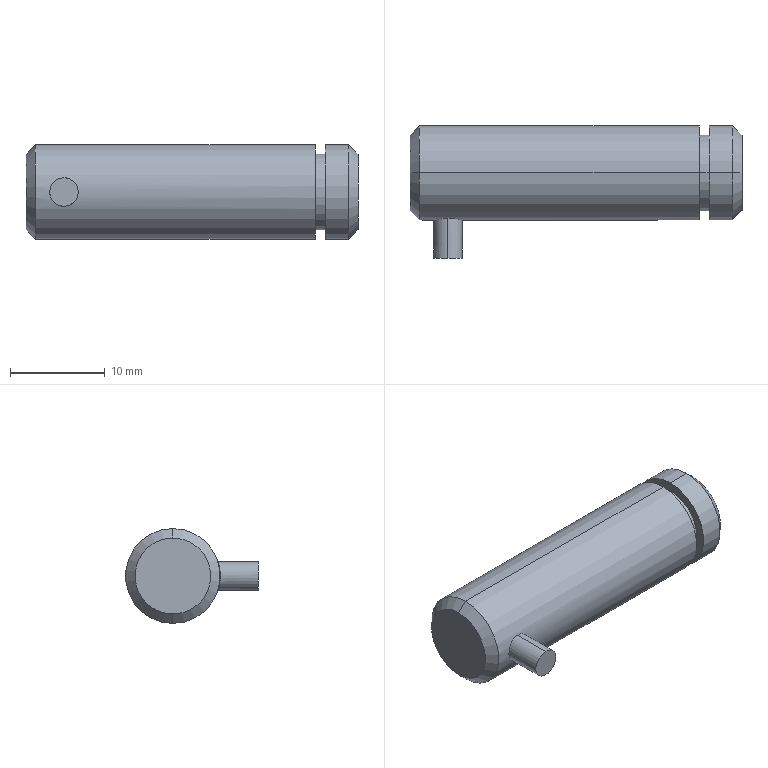Part | SolidWorks | features Revolution 2, Chamfer 1 | 1 solid | 17 faces | box 35 x 14 x 10 mm | volume 2719 mm3 | cylinder 8 | plane 5 | cone 4 | commonest cylinder face diameters 10 x4 3 x2 8 x2
STEP:
#1=CARTESIAN_POINT('',(17.5,0.,-4.));
#2=VERTEX_POINT('',#1);
#3=CARTESIAN_POINT('',(17.5,0.,4.));
#4=VERTEX_POINT('',#3);
#5=CARTESIAN_POINT('',(17.5,0.,0.));
#6=DIRECTION('',(1.,0.,0.));
#7=DIRECTION('',(0.,0.,-1.));
#8=AXIS2_PLACEMENT_3D('',#5,#6,#7);
#9=CIRCLE('',#8,4.);
#10=EDGE_CURVE('',#2,#4,#9,.T.);
#11=ORIENTED_EDGE('',*,*,#10,.F.);
#12=CARTESIAN_POINT('',(16.5,0.,-5.));
#13=VERTEX_POINT('',#12);
#14=CARTESIAN_POINT('',(16.5,0.,-5.));
#15=DIRECTION('',(-0.7071,0.,-0.7071));
#16=VECTOR('',#15,1000.);
#17=LINE('',#14,#16);
#18=EDGE_CURVE('',#2,#13,#17,.T.);
#19=ORIENTED_EDGE('',*,*,#18,.T.);
#20=CARTESIAN_POINT('',(16.5,0.,5.));
#21=VERTEX_POINT('',#20);
#22=CARTESIAN_POINT('',(16.5,0.,0.));
#23=DIRECTION('',(-1.,0.,0.));
#24=DIRECTION('',(0.,0.,-1.));
#25=AXIS2_PLACEMENT_3D('',#22,#23,#24);
#26=CIRCLE('',#25,5.);
#27=EDGE_CURVE('',#21,#13,#26,.T.);
#28=ORIENTED_EDGE('',*,*,#27,.F.);
#29=CARTESIAN_POINT('',(16.5,0.,5.));
#30=DIRECTION('',(-0.7071,0.,0.7071));
#31=VECTOR('',#30,1000.);
#32=LINE('',#29,#31);
#33=EDGE_CURVE('',#4,#21,#32,.T.);
#34=ORIENTED_EDGE('',*,*,#33,.F.);
#35=EDGE_LOOP('',(#11,#19,#28,#34));
#36=FACE_OUTER_BOUND('',#35,.T.);
#37=CARTESIAN_POINT('',(16.5,0.,0.));
#38=DIRECTION('',(-1.,0.,0.));
#39=DIRECTION('',(0.,0.,1.));
#40=AXIS2_PLACEMENT_3D('',#37,#38,#39);
#41=CONICAL_SURFACE('',#40,5.,0.7854);
#42=ADVANCED_FACE('',(#36),#41,.T.);
#43=CARTESIAN_POINT('',(-17.5,0.,4.));
#44=VERTEX_POINT('',#43);
#45=CARTESIAN_POINT('',(-17.5,0.,-4.));
#46=VERTEX_POINT('',#45);
#47=CARTESIAN_POINT('',(-17.5,0.,0.));
#48=DIRECTION('',(-1.,0.,0.));
#49=DIRECTION('',(0.,0.,1.));
#50=AXIS2_PLACEMENT_3D('',#47,#48,#49);
#51=CIRCLE('',#50,4.);
#52=EDGE_CURVE('',#44,#46,#51,.T.);
#53=ORIENTED_EDGE('',*,*,#52,.F.);
#54=CARTESIAN_POINT('',(-16.5,0.,5.));
#55=VERTEX_POINT('',#54);
#56=CARTESIAN_POINT('',(-17.5,0.,4.));
#57=DIRECTION('',(0.7071,0.,0.7071));
#58=VECTOR('',#57,1000.);
#59=LINE('',#56,#58);
#60=EDGE_CURVE('',#44,#55,#59,.T.);
#61=ORIENTED_EDGE('',*,*,#60,.T.);
#62=CARTESIAN_POINT('',(-16.5,0.,-5.));
#63=VERTEX_POINT('',#62);
#64=CARTESIAN_POINT('',(-16.5,0.,0.));
#65=DIRECTION('',(1.,0.,0.));
#66=DIRECTION('',(0.,0.,1.));
#67=AXIS2_PLACEMENT_3D('',#64,#65,#66);
#68=CIRCLE('',#67,5.);
#69=EDGE_CURVE('',#63,#55,#68,.T.);
#70=ORIENTED_EDGE('',*,*,#69,.F.);
#71=CARTESIAN_POINT('',(-17.5,0.,-4.));
#72=DIRECTION('',(0.7071,0.,-0.7071));
#73=VECTOR('',#72,1000.);
#74=LINE('',#71,#73);
#75=EDGE_CURVE('',#46,#63,#74,.T.);
#76=ORIENTED_EDGE('',*,*,#75,.F.);
#77=EDGE_LOOP('',(#53,#61,#70,#76));
#78=FACE_OUTER_BOUND('',#77,.T.);
#79=CARTESIAN_POINT('',(-17.5,0.,0.));
#80=DIRECTION('',(1.,0.,0.));
#81=DIRECTION('',(0.,0.,-1.));
#82=AXIS2_PLACEMENT_3D('',#79,#80,#81);
#83=CONICAL_SURFACE('',#82,4.,0.7854);
#84=ADVANCED_FACE('',(#78),#83,.T.);
#85=CARTESIAN_POINT('',(-13.5,-4.77,-1.5));
#86=VERTEX_POINT('',#85);
#87=CARTESIAN_POINT('',(-13.5,-4.77,1.5));
#88=VERTEX_POINT('',#87);
#89=CARTESIAN_POINT('',(-13.5,-4.77,-1.5));
#90=CARTESIAN_POINT('',(-13.4,-4.77,-1.5));
#91=CARTESIAN_POINT('',(-13.302,-4.773,-1.49));
#92=CARTESIAN_POINT('',(-13.11,-4.785,-1.452));
#93=CARTESIAN_POINT('',(-13.014,-4.794,-1.423));
#94=CARTESIAN_POINT('',(-12.833,-4.815,-1.347));
#95=CARTESIAN_POINT('',(-12.747,-4.828,-1.301));
#96=CARTESIAN_POINT('',(-12.584,-4.856,-1.192));
#97=CARTESIAN_POINT('',(-12.508,-4.871,-1.129));
#98=CARTESIAN_POINT('',(-12.302,-4.916,-0.9229));
#99=CARTESIAN_POINT('',(-12.19,-4.946,-0.7565));
#100=CARTESIAN_POINT('',(-12.04,-4.988,-0.3958));
#101=CARTESIAN_POINT('',(-12.,-5.,-0.1976));
#102=CARTESIAN_POINT('',(-12.,-5.,0.09784));
#103=CARTESIAN_POINT('',(-12.01,-4.997,0.1979));
#104=CARTESIAN_POINT('',(-12.048,-4.986,0.3908));
#105=CARTESIAN_POINT('',(-12.077,-4.977,0.4846));
#106=CARTESIAN_POINT('',(-12.191,-4.946,0.7582));
#107=CARTESIAN_POINT('',(-12.301,-4.916,0.9228));
#108=CARTESIAN_POINT('',(-12.509,-4.871,1.13));
#109=CARTESIAN_POINT('',(-12.584,-4.856,1.192));
#110=CARTESIAN_POINT('',(-12.746,-4.828,1.301));
#111=CARTESIAN_POINT('',(-12.834,-4.815,1.348));
#112=CARTESIAN_POINT('',(-13.015,-4.793,1.423));
#113=CARTESIAN_POINT('',(-13.108,-4.785,1.451));
#114=CARTESIAN_POINT('',(-13.302,-4.773,1.49));
#115=CARTESIAN_POINT('',(-13.402,-4.77,1.5));
#116=CARTESIAN_POINT('',(-13.5,-4.77,1.5));
#117=B_SPLINE_CURVE_WITH_KNOTS('',3,(#89,#90,#91,#92,#93,#94,#95,#96,#97,#98,#99,#100,#101,#102,#103,#104,#105,#106,#107,#108,#109,#110,#111,#112,#113,#114,#115,#116),.UNSPECIFIED.,.F.,.F.,(4,2,2,2,2,2,2,2,2,2,2,2,2,4),(0.,0.0002948,0.0005896,0.0008844,0.001179,0.001769,0.002358,0.002653,0.002948,0.003538,0.003833,0.004127,0.004422,0.004717),.UNSPECIFIED.);
#118=EDGE_CURVE('',#86,#88,#117,.T.);
#119=ORIENTED_EDGE('',*,*,#118,.T.);
#120=CARTESIAN_POINT('',(-13.5,-9.,1.5));
#121=VERTEX_POINT('',#120);
#122=CARTESIAN_POINT('',(-13.5,-4.77,1.5));
#123=DIRECTION('',(0.,-1.,0.));
#124=VECTOR('',#123,1000.);
#125=LINE('',#122,#124);
#126=EDGE_CURVE('',#88,#121,#125,.T.);
#127=ORIENTED_EDGE('',*,*,#126,.T.);
#128=CARTESIAN_POINT('',(-13.5,-9.,-1.5));
#129=VERTEX_POINT('',#128);
#130=CARTESIAN_POINT('',(-13.5,-9.,0.));
#131=DIRECTION('',(0.,-1.,0.));
#132=DIRECTION('',(0.,0.,-1.));
#133=AXIS2_PLACEMENT_3D('',#130,#131,#132);
#134=CIRCLE('',#133,1.5);
#135=EDGE_CURVE('',#129,#121,#134,.T.);
#136=ORIENTED_EDGE('',*,*,#135,.F.);
#137=CARTESIAN_POINT('',(-13.5,-4.77,-1.5));
#138=DIRECTION('',(0.,-1.,0.));
#139=VECTOR('',#138,1000.);
#140=LINE('',#137,#139);
#141=EDGE_CURVE('',#86,#129,#140,.T.);
#142=ORIENTED_EDGE('',*,*,#141,.F.);
#143=EDGE_LOOP('',(#119,#127,#136,#142));
#144=FACE_OUTER_BOUND('',#143,.T.);
#145=CARTESIAN_POINT('',(-13.5,-4.77,0.));
#146=DIRECTION('',(0.,-1.,0.));
#147=DIRECTION('',(0.,0.,-1.));
#148=AXIS2_PLACEMENT_3D('',#145,#146,#147);
#149=CYLINDRICAL_SURFACE('',#148,1.5);
#150=ADVANCED_FACE('',(#144),#149,.T.);
#151=CARTESIAN_POINT('',(14.05,0.,4.));
#152=VERTEX_POINT('',#151);
#153=CARTESIAN_POINT('',(14.05,0.,-4.));
#154=VERTEX_POINT('',#153);
#155=CARTESIAN_POINT('',(14.05,0.,0.));
#156=DIRECTION('',(-1.,0.,0.));
#157=DIRECTION('',(0.,0.,1.));
#158=AXIS2_PLACEMENT_3D('',#155,#156,#157);
#159=CIRCLE('',#158,4.);
#160=EDGE_CURVE('',#152,#154,#159,.T.);
#161=ORIENTED_EDGE('',*,*,#160,.T.);
#162=CARTESIAN_POINT('',(13.,0.,-4.));
#163=VERTEX_POINT('',#162);
#164=CARTESIAN_POINT('',(17.5,0.,-4.));
#165=DIRECTION('',(-1.,0.,0.));
#166=VECTOR('',#165,1000.);
#167=LINE('',#164,#166);
#168=EDGE_CURVE('',#154,#163,#167,.T.);
#169=ORIENTED_EDGE('',*,*,#168,.T.);
#170=CARTESIAN_POINT('',(13.,0.,4.));
#171=VERTEX_POINT('',#170);
#172=CARTESIAN_POINT('',(13.,0.,0.));
#173=DIRECTION('',(-1.,0.,0.));
#174=DIRECTION('',(0.,0.,1.));
#175=AXIS2_PLACEMENT_3D('',#172,#173,#174);
#176=CIRCLE('',#175,4.);
#177=EDGE_CURVE('',#171,#163,#176,.T.);
#178=ORIENTED_EDGE('',*,*,#177,.F.);
#179=CARTESIAN_POINT('',(17.5,0.,4.));
#180=DIRECTION('',(-1.,0.,0.));
#181=VECTOR('',#180,1000.);
#182=LINE('',#179,#181);
#183=EDGE_CURVE('',#152,#171,#182,.T.);
#184=ORIENTED_EDGE('',*,*,#183,.F.);
#185=EDGE_LOOP('',(#161,#169,#178,#184));
#186=FACE_OUTER_BOUND('',#185,.T.);
#187=CARTESIAN_POINT('',(17.5,0.,0.));
#188=DIRECTION('',(-1.,0.,0.));
#189=DIRECTION('',(0.,0.,1.));
#190=AXIS2_PLACEMENT_3D('',#187,#188,#189);
#191=CYLINDRICAL_SURFACE('',#190,4.);
#192=ADVANCED_FACE('',(#186),#191,.T.);
#193=CARTESIAN_POINT('',(13.,0.,5.));
#194=VERTEX_POINT('',#193);
#195=CARTESIAN_POINT('',(13.,0.,-5.));
#196=VERTEX_POINT('',#195);
#197=CARTESIAN_POINT('',(13.,0.,0.));
#198=DIRECTION('',(-1.,0.,0.));
#199=DIRECTION('',(0.,0.,1.));
#200=AXIS2_PLACEMENT_3D('',#197,#198,#199);
#201=CIRCLE('',#200,5.);
#202=EDGE_CURVE('',#194,#196,#201,.T.);
#203=ORIENTED_EDGE('',*,*,#202,.T.);
#204=CARTESIAN_POINT('',(17.5,0.,-5.));
#205=DIRECTION('',(-1.,0.,0.));
#206=VECTOR('',#205,1000.);
#207=LINE('',#204,#206);
#208=EDGE_CURVE('',#196,#63,#207,.T.);
#209=ORIENTED_EDGE('',*,*,#208,.T.);
#210=ORIENTED_EDGE('',*,*,#69,.T.);
#211=CARTESIAN_POINT('',(17.5,0.,5.));
#212=DIRECTION('',(-1.,0.,0.));
#213=VECTOR('',#212,1000.);
#214=LINE('',#211,#213);
#215=EDGE_CURVE('',#194,#55,#214,.T.);
#216=ORIENTED_EDGE('',*,*,#215,.F.);
#217=EDGE_LOOP('',(#203,#209,#210,#216));
#218=FACE_OUTER_BOUND('',#217,.T.);
#219=CARTESIAN_POINT('',(17.5,0.,0.));
#220=DIRECTION('',(-1.,0.,0.));
#221=DIRECTION('',(0.,0.,1.));
#222=AXIS2_PLACEMENT_3D('',#219,#220,#221);
#223=CYLINDRICAL_SURFACE('',#222,5.);
#224=ADVANCED_FACE('',(#218),#223,.T.);
#225=ORIENTED_EDGE('',*,*,#27,.T.);
#226=CARTESIAN_POINT('',(14.05,0.,-5.));
#227=VERTEX_POINT('',#226);
#228=CARTESIAN_POINT('',(17.5,0.,-5.));
#229=DIRECTION('',(-1.,0.,0.));
#230=VECTOR('',#229,1000.);
#231=LINE('',#228,#230);
#232=EDGE_CURVE('',#13,#227,#231,.T.);
#233=ORIENTED_EDGE('',*,*,#232,.T.);
#234=CARTESIAN_POINT('',(14.05,0.,5.));
#235=VERTEX_POINT('',#234);
#236=CARTESIAN_POINT('',(14.05,0.,0.));
#237=DIRECTION('',(-1.,0.,0.));
#238=DIRECTION('',(0.,0.,1.));
#239=AXIS2_PLACEMENT_3D('',#236,#237,#238);
#240=CIRCLE('',#239,5.);
#241=EDGE_CURVE('',#235,#227,#240,.T.);
#242=ORIENTED_EDGE('',*,*,#241,.F.);
#243=CARTESIAN_POINT('',(17.5,0.,5.));
#244=DIRECTION('',(-1.,0.,0.));
#245=VECTOR('',#244,1000.);
#246=LINE('',#243,#245);
#247=EDGE_CURVE('',#21,#235,#246,.T.);
#248=ORIENTED_EDGE('',*,*,#247,.F.);
#249=EDGE_LOOP('',(#225,#233,#242,#248));
#250=FACE_OUTER_BOUND('',#249,.T.);
#251=CARTESIAN_POINT('',(17.5,0.,0.));
#252=DIRECTION('',(-1.,0.,0.));
#253=DIRECTION('',(0.,0.,1.));
#254=AXIS2_PLACEMENT_3D('',#251,#252,#253);
#255=CYLINDRICAL_SURFACE('',#254,5.);
#256=ADVANCED_FACE('',(#250),#255,.T.);
#257=ORIENTED_EDGE('',*,*,#232,.F.);
#258=CARTESIAN_POINT('',(16.5,0.,0.));
#259=DIRECTION('',(-1.,0.,0.));
#260=DIRECTION('',(0.,0.,-1.));
#261=AXIS2_PLACEMENT_3D('',#258,#259,#260);
#262=CIRCLE('',#261,5.);
#263=EDGE_CURVE('',#13,#21,#262,.T.);
#264=ORIENTED_EDGE('',*,*,#263,.T.);
#265=ORIENTED_EDGE('',*,*,#247,.T.);
#266=CARTESIAN_POINT('',(14.05,0.,0.));
#267=DIRECTION('',(-1.,0.,0.));
#268=DIRECTION('',(0.,0.,1.));
#269=AXIS2_PLACEMENT_3D('',#266,#267,#268);
#270=CIRCLE('',#269,5.);
#271=EDGE_CURVE('',#227,#235,#270,.T.);
#272=ORIENTED_EDGE('',*,*,#271,.F.);
#273=EDGE_LOOP('',(#257,#264,#265,#272));
#274=FACE_OUTER_BOUND('',#273,.T.);
#275=CARTESIAN_POINT('',(17.5,0.,0.));
#276=DIRECTION('',(-1.,0.,0.));
#277=DIRECTION('',(0.,0.,1.));
#278=AXIS2_PLACEMENT_3D('',#275,#276,#277);
#279=CYLINDRICAL_SURFACE('',#278,5.);
#280=ADVANCED_FACE('',(#274),#279,.T.);
#281=CARTESIAN_POINT('',(17.5,0.,0.));
#282=DIRECTION('',(1.,0.,0.));
#283=DIRECTION('',(0.,0.,-1.));
#284=AXIS2_PLACEMENT_3D('',#281,#282,#283);
#285=CIRCLE('',#284,4.);
#286=EDGE_CURVE('',#4,#2,#285,.T.);
#287=ORIENTED_EDGE('',*,*,#286,.T.);
#288=ORIENTED_EDGE('',*,*,#10,.T.);
#289=EDGE_LOOP('',(#287,#288));
#290=FACE_OUTER_BOUND('',#289,.T.);
#291=CARTESIAN_POINT('',(17.5,5.,0.));
#292=DIRECTION('',(1.,0.,0.));
#293=DIRECTION('',(0.,0.,-1.));
#294=AXIS2_PLACEMENT_3D('',#291,#292,#293);
#295=PLANE('',#294);
#296=ADVANCED_FACE('',(#290),#295,.T.);
#297=CARTESIAN_POINT('',(-17.5,0.,0.));
#298=DIRECTION('',(-1.,0.,0.));
#299=DIRECTION('',(0.,0.,1.));
#300=AXIS2_PLACEMENT_3D('',#297,#298,#299);
#301=CIRCLE('',#300,4.);
#302=EDGE_CURVE('',#46,#44,#301,.T.);
#303=ORIENTED_EDGE('',*,*,#302,.T.);
#304=ORIENTED_EDGE('',*,*,#52,.T.);
#305=EDGE_LOOP('',(#303,#304));
#306=FACE_OUTER_BOUND('',#305,.T.);
#307=CARTESIAN_POINT('',(-17.5,0.,0.));
#308=DIRECTION('',(-1.,0.,0.));
#309=DIRECTION('',(0.,0.,1.));
#310=AXIS2_PLACEMENT_3D('',#307,#308,#309);
#311=PLANE('',#310);
#312=ADVANCED_FACE('',(#306),#311,.T.);
#313=ORIENTED_EDGE('',*,*,#208,.F.);
#314=CARTESIAN_POINT('',(13.,0.,0.));
#315=DIRECTION('',(-1.,0.,0.));
#316=DIRECTION('',(0.,0.,1.));
#317=AXIS2_PLACEMENT_3D('',#314,#315,#316);
#318=CIRCLE('',#317,5.);
#319=EDGE_CURVE('',#196,#194,#318,.T.);
#320=ORIENTED_EDGE('',*,*,#319,.T.);
#321=ORIENTED_EDGE('',*,*,#215,.T.);
#322=CARTESIAN_POINT('',(-16.5,0.,0.));
#323=DIRECTION('',(1.,0.,0.));
#324=DIRECTION('',(0.,0.,1.));
#325=AXIS2_PLACEMENT_3D('',#322,#323,#324);
#326=CIRCLE('',#325,5.);
#327=EDGE_CURVE('',#55,#63,#326,.T.);
#328=ORIENTED_EDGE('',*,*,#327,.T.);
#329=EDGE_LOOP('',(#313,#320,#321,#328));
#330=FACE_OUTER_BOUND('',#329,.T.);
#331=ORIENTED_EDGE('',*,*,#118,.F.);
#332=CARTESIAN_POINT('',(-13.5,-4.77,1.5));
#333=CARTESIAN_POINT('',(-13.696,-4.77,1.5));
#334=CARTESIAN_POINT('',(-13.895,-4.783,1.46));
#335=CARTESIAN_POINT('',(-14.166,-4.815,1.348));
#336=CARTESIAN_POINT('',(-14.254,-4.828,1.301));
#337=CARTESIAN_POINT('',(-14.416,-4.856,1.192));
#338=CARTESIAN_POINT('',(-14.491,-4.871,1.13));
#339=CARTESIAN_POINT('',(-14.699,-4.916,0.9226));
#340=CARTESIAN_POINT('',(-14.809,-4.945,0.759));
#341=CARTESIAN_POINT('',(-14.923,-4.977,0.4847));
#342=CARTESIAN_POINT('',(-14.951,-4.986,0.3909));
#343=CARTESIAN_POINT('',(-14.99,-4.997,0.1986));
#344=CARTESIAN_POINT('',(-15.,-5.,0.09894));
#345=CARTESIAN_POINT('',(-15.,-5.,-0.09877));
#346=CARTESIAN_POINT('',(-14.99,-4.997,-0.1965));
#347=CARTESIAN_POINT('',(-14.952,-4.986,-0.3898));
#348=CARTESIAN_POINT('',(-14.923,-4.977,-0.4855));
#349=CARTESIAN_POINT('',(-14.81,-4.946,-0.7566));
#350=CARTESIAN_POINT('',(-14.698,-4.916,-0.9229));
#351=CARTESIAN_POINT('',(-14.492,-4.871,-1.129));
#352=CARTESIAN_POINT('',(-14.416,-4.856,-1.192));
#353=CARTESIAN_POINT('',(-14.253,-4.828,-1.301));
#354=CARTESIAN_POINT('',(-14.167,-4.815,-1.347));
#355=CARTESIAN_POINT('',(-13.986,-4.794,-1.422));
#356=CARTESIAN_POINT('',(-13.891,-4.785,-1.452));
#357=CARTESIAN_POINT('',(-13.698,-4.773,-1.49));
#358=CARTESIAN_POINT('',(-13.6,-4.77,-1.5));
#359=CARTESIAN_POINT('',(-13.5,-4.77,-1.5));
#360=B_SPLINE_CURVE_WITH_KNOTS('',3,(#332,#333,#334,#335,#336,#337,#338,#339,#340,#341,#342,#343,#344,#345,#346,#347,#348,#349,#350,#351,#352,#353,#354,#355,#356,#357,#358,#359),.UNSPECIFIED.,.F.,.F.,(4,2,2,2,2,2,2,2,2,2,2,2,2,4),(0.004717,0.005306,0.005601,0.005896,0.006485,0.00678,0.007075,0.007369,0.007664,0.008254,0.008548,0.008843,0.009138,0.009433),.UNSPECIFIED.);
#361=EDGE_CURVE('',#88,#86,#360,.T.);
#362=ORIENTED_EDGE('',*,*,#361,.F.);
#363=EDGE_LOOP('',(#331,#362));
#364=FACE_BOUND('',#363,.T.);
#365=CARTESIAN_POINT('',(17.5,0.,0.));
#366=DIRECTION('',(-1.,0.,0.));
#367=DIRECTION('',(0.,0.,1.));
#368=AXIS2_PLACEMENT_3D('',#365,#366,#367);
#369=CYLINDRICAL_SURFACE('',#368,5.);
#370=ADVANCED_FACE('',(#330,#364),#369,.T.);
#371=ORIENTED_EDGE('',*,*,#177,.T.);
#372=CARTESIAN_POINT('',(13.,0.,0.));
#373=DIRECTION('',(-1.,0.,0.));
#374=DIRECTION('',(0.,0.,1.));
#375=AXIS2_PLACEMENT_3D('',#372,#373,#374);
#376=CIRCLE('',#375,4.);
#377=EDGE_CURVE('',#163,#171,#376,.T.);
#378=ORIENTED_EDGE('',*,*,#377,.T.);
#379=EDGE_LOOP('',(#371,#378));
#380=FACE_BOUND('',#379,.T.);
#381=ORIENTED_EDGE('',*,*,#202,.F.);
#382=ORIENTED_EDGE('',*,*,#319,.F.);
#383=EDGE_LOOP('',(#381,#382));
#384=FACE_OUTER_BOUND('',#383,.T.);
#385=CARTESIAN_POINT('',(13.,5.,0.));
#386=DIRECTION('',(1.,0.,0.));
#387=DIRECTION('',(0.,0.,-1.));
#388=AXIS2_PLACEMENT_3D('',#385,#386,#387);
#389=PLANE('',#388);
#390=ADVANCED_FACE('',(#380,#384),#389,.T.);
#391=ORIENTED_EDGE('',*,*,#168,.F.);
#392=CARTESIAN_POINT('',(14.05,0.,0.));
#393=DIRECTION('',(-1.,0.,0.));
#394=DIRECTION('',(0.,0.,1.));
#395=AXIS2_PLACEMENT_3D('',#392,#393,#394);
#396=CIRCLE('',#395,4.);
#397=EDGE_CURVE('',#154,#152,#396,.T.);
#398=ORIENTED_EDGE('',*,*,#397,.T.);
#399=ORIENTED_EDGE('',*,*,#183,.T.);
#400=ORIENTED_EDGE('',*,*,#377,.F.);
#401=EDGE_LOOP('',(#391,#398,#399,#400));
#402=FACE_OUTER_BOUND('',#401,.T.);
#403=CARTESIAN_POINT('',(17.5,0.,0.));
#404=DIRECTION('',(-1.,0.,0.));
#405=DIRECTION('',(0.,0.,1.));
#406=AXIS2_PLACEMENT_3D('',#403,#404,#405);
#407=CYLINDRICAL_SURFACE('',#406,4.);
#408=ADVANCED_FACE('',(#402),#407,.T.);
#409=ORIENTED_EDGE('',*,*,#241,.T.);
#410=ORIENTED_EDGE('',*,*,#271,.T.);
#411=EDGE_LOOP('',(#409,#410));
#412=FACE_OUTER_BOUND('',#411,.T.);
#413=ORIENTED_EDGE('',*,*,#160,.F.);
#414=ORIENTED_EDGE('',*,*,#397,.F.);
#415=EDGE_LOOP('',(#413,#414));
#416=FACE_BOUND('',#415,.T.);
#417=CARTESIAN_POINT('',(14.05,4.,0.));
#418=DIRECTION('',(-1.,0.,0.));
#419=DIRECTION('',(0.,0.,1.));
#420=AXIS2_PLACEMENT_3D('',#417,#418,#419);
#421=PLANE('',#420);
#422=ADVANCED_FACE('',(#412,#416),#421,.T.);
#423=ORIENTED_EDGE('',*,*,#135,.T.);
#424=CARTESIAN_POINT('',(-13.5,-9.,0.));
#425=DIRECTION('',(0.,-1.,0.));
#426=DIRECTION('',(0.,0.,-1.));
#427=AXIS2_PLACEMENT_3D('',#424,#425,#426);
#428=CIRCLE('',#427,1.5);
#429=EDGE_CURVE('',#121,#129,#428,.T.);
#430=ORIENTED_EDGE('',*,*,#429,.T.);
#431=EDGE_LOOP('',(#423,#430));
#432=FACE_OUTER_BOUND('',#431,.T.);
#433=CARTESIAN_POINT('',(-13.5,-9.,0.));
#434=DIRECTION('',(0.,-1.,0.));
#435=DIRECTION('',(0.,0.,-1.));
#436=AXIS2_PLACEMENT_3D('',#433,#434,#435);
#437=PLANE('',#436);
#438=ADVANCED_FACE('',(#432),#437,.T.);
#439=ORIENTED_EDGE('',*,*,#126,.F.);
#440=ORIENTED_EDGE('',*,*,#361,.T.);
#441=ORIENTED_EDGE('',*,*,#141,.T.);
#442=ORIENTED_EDGE('',*,*,#429,.F.);
#443=EDGE_LOOP('',(#439,#440,#441,#442));
#444=FACE_OUTER_BOUND('',#443,.T.);
#445=CARTESIAN_POINT('',(-13.5,-4.77,0.));
#446=DIRECTION('',(0.,-1.,0.));
#447=DIRECTION('',(0.,0.,-1.));
#448=AXIS2_PLACEMENT_3D('',#445,#446,#447);
#449=CYLINDRICAL_SURFACE('',#448,1.5);
#450=ADVANCED_FACE('',(#444),#449,.T.);
#451=ORIENTED_EDGE('',*,*,#60,.F.);
#452=ORIENTED_EDGE('',*,*,#302,.F.);
#453=ORIENTED_EDGE('',*,*,#75,.T.);
#454=ORIENTED_EDGE('',*,*,#327,.F.);
#455=EDGE_LOOP('',(#451,#452,#453,#454));
#456=FACE_OUTER_BOUND('',#455,.T.);
#457=CARTESIAN_POINT('',(-17.5,0.,0.));
#458=DIRECTION('',(1.,0.,0.));
#459=DIRECTION('',(0.,0.,-1.));
#460=AXIS2_PLACEMENT_3D('',#457,#458,#459);
#461=CONICAL_SURFACE('',#460,4.,0.7854);
#462=ADVANCED_FACE('',(#456),#461,.T.);
#463=ORIENTED_EDGE('',*,*,#18,.F.);
#464=ORIENTED_EDGE('',*,*,#286,.F.);
#465=ORIENTED_EDGE('',*,*,#33,.T.);
#466=ORIENTED_EDGE('',*,*,#263,.F.);
#467=EDGE_LOOP('',(#463,#464,#465,#466));
#468=FACE_OUTER_BOUND('',#467,.T.);
#469=CARTESIAN_POINT('',(16.5,0.,0.));
#470=DIRECTION('',(-1.,0.,0.));
#471=DIRECTION('',(0.,0.,1.));
#472=AXIS2_PLACEMENT_3D('',#469,#470,#471);
#473=CONICAL_SURFACE('',#472,5.,0.7854);
#474=ADVANCED_FACE('',(#468),#473,.T.);
#475=CLOSED_SHELL('',(#42,#84,#150,#192,#224,#256,#280,#296,#312,#370,#390,#408,#422,#438,#450,#462,#474));
#476=MANIFOLD_SOLID_BREP('',#475);
#477=CARTESIAN_POINT('',(0.,0.,0.));
#478=DIRECTION('',(0.,0.,1.));
#479=DIRECTION('',(1.,0.,0.));
#480=AXIS2_PLACEMENT_3D('',#477,#478,#479);
#481=(LENGTH_UNIT()NAMED_UNIT(*)SI_UNIT(.MILLI.,.METRE.));
#482=UNCERTAINTY_MEASURE_WITH_UNIT(LENGTH_MEASURE(0.00001),#481,'','');
#483=(NAMED_UNIT(*)PLANE_ANGLE_UNIT()SI_UNIT($,.RADIAN.));
#484=(NAMED_UNIT(*)SI_UNIT($,.STERADIAN.)SOLID_ANGLE_UNIT());
#485=(GEOMETRIC_REPRESENTATION_CONTEXT(3)GLOBAL_UNCERTAINTY_ASSIGNED_CONTEXT((#482))GLOBAL_UNIT_ASSIGNED_CONTEXT((#481,#483,#484))REPRESENTATION_CONTEXT('',''));
#486=ADVANCED_BREP_SHAPE_REPRESENTATION('',(#476,#480),#485);